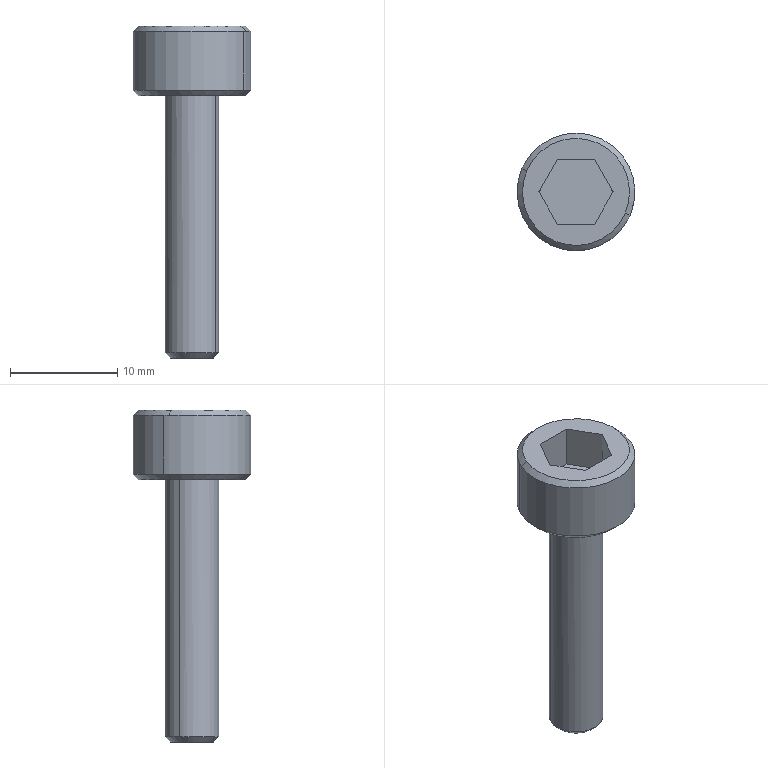Part | STEP file | Bolt.12A.stp | 1 solid | 20 faces | box 11 x 11 x 31 mm | volume 963.854 mm3 | plane 10 | cone 6 | cylinder 4 | commonest cylinder face diameters 5 x2 11 x2
STEP:
#1=CARTESIAN_POINT('',(0.,0.,0.));
#2=DIRECTION('',(0.,0.,1.));
#3=DIRECTION('',(1.,0.,0.));
#4=AXIS2_PLACEMENT_3D('',#1,#2,#3);
#5=CARTESIAN_POINT('',(3.464,0.,0.));
#6=VERTEX_POINT('',#5);
#7=CARTESIAN_POINT('',(3.464,0.,-4.));
#8=VERTEX_POINT('',#7);
#9=CARTESIAN_POINT('',(3.464,0.,0.));
#10=DIRECTION('',(0.,0.,-1.));
#11=VECTOR('',#10,1.);
#12=LINE('',#9,#11);
#13=CARTESIAN_POINT('',(3.551,-0.15,0.2));
#14=DIRECTION('',(-0.866,-0.5,0.));
#15=DIRECTION('',(-0.5,0.866,0.));
#16=AXIS2_PLACEMENT_3D('',#13,#14,#15);
#17=PLANE('',#16);
#18=CARTESIAN_POINT('',(0.1732,0.2));
#19=DIRECTION('',(0.,1.));
#20=VECTOR('',#19,1.);
#21=LINE('',#18,#20);
#22=(GEOMETRIC_REPRESENTATION_CONTEXT(2)PARAMETRIC_REPRESENTATION_CONTEXT()REPRESENTATION_CONTEXT('',''));
#23=DEFINITIONAL_REPRESENTATION('',(#21),#22);
#24=PCURVE('',#17,#23);
#25=CARTESIAN_POINT('',(1.645,-3.15,-4.2));
#26=DIRECTION('',(-0.866,0.5,0.));
#27=DIRECTION('',(0.,0.,1.));
#28=AXIS2_PLACEMENT_3D('',#25,#26,#27);
#29=PLANE('',#28);
#30=CARTESIAN_POINT('',(4.2,3.637));
#31=DIRECTION('',(-1.,0.));
#32=VECTOR('',#31,1.);
#33=LINE('',#30,#32);
#34=(GEOMETRIC_REPRESENTATION_CONTEXT(2)PARAMETRIC_REPRESENTATION_CONTEXT()REPRESENTATION_CONTEXT('',''));
#35=DEFINITIONAL_REPRESENTATION('',(#33),#34);
#36=PCURVE('',#29,#35);
#37=SURFACE_CURVE('',#12,(#24,#36),.PCURVE_S1.);
#38=EDGE_CURVE('',#6,#8,#37,.T.);
#39=ORIENTED_EDGE('',*,*,#38,.F.);
#40=CARTESIAN_POINT('',(1.732,3.,0.));
#41=VERTEX_POINT('',#40);
#42=CARTESIAN_POINT('',(3.464,0.,0.));
#43=DIRECTION('',(-0.5,0.866,0.));
#44=VECTOR('',#43,1.);
#45=LINE('',#42,#44);
#46=CARTESIAN_POINT('',(0.1732,0.2));
#47=DIRECTION('',(1.,0.));
#48=VECTOR('',#47,1.);
#49=LINE('',#46,#48);
#50=(GEOMETRIC_REPRESENTATION_CONTEXT(2)PARAMETRIC_REPRESENTATION_CONTEXT()REPRESENTATION_CONTEXT('',''));
#51=DEFINITIONAL_REPRESENTATION('',(#49),#50);
#52=PCURVE('',#17,#51);
#53=CARTESIAN_POINT('',(5.5,5.5,0.));
#54=DIRECTION('',(0.,0.,-1.));
#55=DIRECTION('',(0.,-1.,0.));
#56=AXIS2_PLACEMENT_3D('',#53,#54,#55);
#57=PLANE('',#56);
#58=CARTESIAN_POINT('',(5.5,2.036));
#59=DIRECTION('',(-0.866,0.5));
#60=VECTOR('',#59,1.);
#61=LINE('',#58,#60);
#62=(GEOMETRIC_REPRESENTATION_CONTEXT(2)PARAMETRIC_REPRESENTATION_CONTEXT()REPRESENTATION_CONTEXT('',''));
#63=DEFINITIONAL_REPRESENTATION('',(#61),#62);
#64=PCURVE('',#57,#63);
#65=SURFACE_CURVE('',#45,(#52,#64),.PCURVE_S1.);
#66=EDGE_CURVE('',#6,#41,#65,.T.);
#67=ORIENTED_EDGE('',*,*,#66,.T.);
#68=CARTESIAN_POINT('',(1.732,3.,-4.));
#69=VERTEX_POINT('',#68);
#70=CARTESIAN_POINT('',(1.732,3.,0.));
#71=DIRECTION('',(0.,0.,-1.));
#72=VECTOR('',#71,1.);
#73=LINE('',#70,#72);
#74=CARTESIAN_POINT('',(3.637,0.2));
#75=DIRECTION('',(0.,1.));
#76=VECTOR('',#75,1.);
#77=LINE('',#74,#76);
#78=(GEOMETRIC_REPRESENTATION_CONTEXT(2)PARAMETRIC_REPRESENTATION_CONTEXT()REPRESENTATION_CONTEXT('',''));
#79=DEFINITIONAL_REPRESENTATION('',(#77),#78);
#80=PCURVE('',#17,#79);
#81=CARTESIAN_POINT('',(-1.905,3.,0.2));
#82=DIRECTION('',(0.,-1.,0.));
#83=DIRECTION('',(0.,0.,-1.));
#84=AXIS2_PLACEMENT_3D('',#81,#82,#83);
#85=PLANE('',#84);
#86=CARTESIAN_POINT('',(0.2,3.637));
#87=DIRECTION('',(1.,0.));
#88=VECTOR('',#87,1.);
#89=LINE('',#86,#88);
#90=(GEOMETRIC_REPRESENTATION_CONTEXT(2)PARAMETRIC_REPRESENTATION_CONTEXT()REPRESENTATION_CONTEXT('',''));
#91=DEFINITIONAL_REPRESENTATION('',(#89),#90);
#92=PCURVE('',#85,#91);
#93=SURFACE_CURVE('',#73,(#80,#92),.PCURVE_S1.);
#94=EDGE_CURVE('',#41,#69,#93,.T.);
#95=ORIENTED_EDGE('',*,*,#94,.T.);
#96=CARTESIAN_POINT('',(3.464,0.,-4.));
#97=DIRECTION('',(-0.5,0.866,0.));
#98=VECTOR('',#97,1.);
#99=LINE('',#96,#98);
#100=CARTESIAN_POINT('',(0.1732,4.2));
#101=DIRECTION('',(1.,0.));
#102=VECTOR('',#101,1.);
#103=LINE('',#100,#102);
#104=(GEOMETRIC_REPRESENTATION_CONTEXT(2)PARAMETRIC_REPRESENTATION_CONTEXT()REPRESENTATION_CONTEXT('',''));
#105=DEFINITIONAL_REPRESENTATION('',(#103),#104);
#106=PCURVE('',#17,#105);
#107=CARTESIAN_POINT('',(-3.811,-3.3,-4.));
#108=DIRECTION('',(0.,0.,1.));
#109=DIRECTION('',(1.,0.,0.));
#110=AXIS2_PLACEMENT_3D('',#107,#108,#109);
#111=PLANE('',#110);
#112=CARTESIAN_POINT('',(7.275,3.3));
#113=DIRECTION('',(-0.5,0.866));
#114=VECTOR('',#113,1.);
#115=LINE('',#112,#114);
#116=(GEOMETRIC_REPRESENTATION_CONTEXT(2)PARAMETRIC_REPRESENTATION_CONTEXT()REPRESENTATION_CONTEXT('',''));
#117=DEFINITIONAL_REPRESENTATION('',(#115),#116);
#118=PCURVE('',#111,#117);
#119=SURFACE_CURVE('',#99,(#106,#118),.PCURVE_S1.);
#120=EDGE_CURVE('',#8,#69,#119,.T.);
#121=ORIENTED_EDGE('',*,*,#120,.F.);
#122=EDGE_LOOP('',(#39,#67,#95,#121));
#123=FACE_BOUND('',#122,.T.);
#124=ADVANCED_FACE('',(#123),#17,.T.);
#125=CARTESIAN_POINT('',(-1.732,3.,0.));
#126=VERTEX_POINT('',#125);
#127=CARTESIAN_POINT('',(-1.732,3.,-4.));
#128=VERTEX_POINT('',#127);
#129=CARTESIAN_POINT('',(-1.732,3.,0.));
#130=DIRECTION('',(0.,0.,-1.));
#131=VECTOR('',#130,1.);
#132=LINE('',#129,#131);
#133=CARTESIAN_POINT('',(-3.551,-0.15,0.2));
#134=DIRECTION('',(0.866,-0.5,0.));
#135=DIRECTION('',(0.,0.,-1.));
#136=AXIS2_PLACEMENT_3D('',#133,#134,#135);
#137=PLANE('',#136);
#138=CARTESIAN_POINT('',(0.2,3.637));
#139=DIRECTION('',(1.,0.));
#140=VECTOR('',#139,1.);
#141=LINE('',#138,#140);
#142=(GEOMETRIC_REPRESENTATION_CONTEXT(2)PARAMETRIC_REPRESENTATION_CONTEXT()REPRESENTATION_CONTEXT('',''));
#143=DEFINITIONAL_REPRESENTATION('',(#141),#142);
#144=PCURVE('',#137,#143);
#145=CARTESIAN_POINT('',(0.2,0.1732));
#146=DIRECTION('',(1.,0.));
#147=VECTOR('',#146,1.);
#148=LINE('',#145,#147);
#149=(GEOMETRIC_REPRESENTATION_CONTEXT(2)PARAMETRIC_REPRESENTATION_CONTEXT()REPRESENTATION_CONTEXT('',''));
#150=DEFINITIONAL_REPRESENTATION('',(#148),#149);
#151=PCURVE('',#85,#150);
#152=SURFACE_CURVE('',#132,(#144,#151),.PCURVE_S1.);
#153=EDGE_CURVE('',#126,#128,#152,.T.);
#154=ORIENTED_EDGE('',*,*,#153,.F.);
#155=CARTESIAN_POINT('',(-3.464,0.,0.));
#156=VERTEX_POINT('',#155);
#157=CARTESIAN_POINT('',(-1.732,3.,0.));
#158=DIRECTION('',(-0.5,-0.866,0.));
#159=VECTOR('',#158,1.);
#160=LINE('',#157,#159);
#161=CARTESIAN_POINT('',(0.2,3.637));
#162=DIRECTION('',(0.,-1.));
#163=VECTOR('',#162,1.);
#164=LINE('',#161,#163);
#165=(GEOMETRIC_REPRESENTATION_CONTEXT(2)PARAMETRIC_REPRESENTATION_CONTEXT()REPRESENTATION_CONTEXT('',''));
#166=DEFINITIONAL_REPRESENTATION('',(#164),#165);
#167=PCURVE('',#137,#166);
#168=CARTESIAN_POINT('',(2.5,7.232));
#169=DIRECTION('',(0.866,0.5));
#170=VECTOR('',#169,1.);
#171=LINE('',#168,#170);
#172=(GEOMETRIC_REPRESENTATION_CONTEXT(2)PARAMETRIC_REPRESENTATION_CONTEXT()REPRESENTATION_CONTEXT('',''));
#173=DEFINITIONAL_REPRESENTATION('',(#171),#172);
#174=PCURVE('',#57,#173);
#175=SURFACE_CURVE('',#160,(#167,#174),.PCURVE_S1.);
#176=EDGE_CURVE('',#126,#156,#175,.T.);
#177=ORIENTED_EDGE('',*,*,#176,.T.);
#178=CARTESIAN_POINT('',(-3.464,0.,-4.));
#179=VERTEX_POINT('',#178);
#180=CARTESIAN_POINT('',(-3.464,0.,0.));
#181=DIRECTION('',(0.,0.,-1.));
#182=VECTOR('',#181,1.);
#183=LINE('',#180,#182);
#184=CARTESIAN_POINT('',(0.2,0.1732));
#185=DIRECTION('',(1.,0.));
#186=VECTOR('',#185,1.);
#187=LINE('',#184,#186);
#188=(GEOMETRIC_REPRESENTATION_CONTEXT(2)PARAMETRIC_REPRESENTATION_CONTEXT()REPRESENTATION_CONTEXT('',''));
#189=DEFINITIONAL_REPRESENTATION('',(#187),#188);
#190=PCURVE('',#137,#189);
#191=CARTESIAN_POINT('',(-1.645,-3.15,0.2));
#192=DIRECTION('',(0.866,0.5,0.));
#193=DIRECTION('',(0.,0.,-1.));
#194=AXIS2_PLACEMENT_3D('',#191,#192,#193);
#195=PLANE('',#194);
#196=CARTESIAN_POINT('',(0.2,3.637));
#197=DIRECTION('',(1.,0.));
#198=VECTOR('',#197,1.);
#199=LINE('',#196,#198);
#200=(GEOMETRIC_REPRESENTATION_CONTEXT(2)PARAMETRIC_REPRESENTATION_CONTEXT()REPRESENTATION_CONTEXT('',''));
#201=DEFINITIONAL_REPRESENTATION('',(#199),#200);
#202=PCURVE('',#195,#201);
#203=SURFACE_CURVE('',#183,(#190,#202),.PCURVE_S1.);
#204=EDGE_CURVE('',#156,#179,#203,.T.);
#205=ORIENTED_EDGE('',*,*,#204,.T.);
#206=CARTESIAN_POINT('',(-1.732,3.,-4.));
#207=DIRECTION('',(-0.5,-0.866,0.));
#208=VECTOR('',#207,1.);
#209=LINE('',#206,#208);
#210=CARTESIAN_POINT('',(4.2,3.637));
#211=DIRECTION('',(0.,-1.));
#212=VECTOR('',#211,1.);
#213=LINE('',#210,#212);
#214=(GEOMETRIC_REPRESENTATION_CONTEXT(2)PARAMETRIC_REPRESENTATION_CONTEXT()REPRESENTATION_CONTEXT('',''));
#215=DEFINITIONAL_REPRESENTATION('',(#213),#214);
#216=PCURVE('',#137,#215);
#217=CARTESIAN_POINT('',(2.078,6.3));
#218=DIRECTION('',(-0.5,-0.866));
#219=VECTOR('',#218,1.);
#220=LINE('',#217,#219);
#221=(GEOMETRIC_REPRESENTATION_CONTEXT(2)PARAMETRIC_REPRESENTATION_CONTEXT()REPRESENTATION_CONTEXT('',''));
#222=DEFINITIONAL_REPRESENTATION('',(#220),#221);
#223=PCURVE('',#111,#222);
#224=SURFACE_CURVE('',#209,(#216,#223),.PCURVE_S1.);
#225=EDGE_CURVE('',#128,#179,#224,.T.);
#226=ORIENTED_EDGE('',*,*,#225,.F.);
#227=EDGE_LOOP('',(#154,#177,#205,#226));
#228=FACE_BOUND('',#227,.T.);
#229=ADVANCED_FACE('',(#228),#137,.T.);
#230=CARTESIAN_POINT('',(-1.732,-3.,-4.));
#231=VERTEX_POINT('',#230);
#232=CARTESIAN_POINT('',(1.732,-3.,-4.));
#233=VERTEX_POINT('',#232);
#234=CARTESIAN_POINT('',(-1.732,-3.,-4.));
#235=DIRECTION('',(1.,0.,0.));
#236=VECTOR('',#235,1.);
#237=LINE('',#234,#236);
#238=CARTESIAN_POINT('',(2.078,0.3));
#239=DIRECTION('',(1.,0.));
#240=VECTOR('',#239,1.);
#241=LINE('',#238,#240);
#242=(GEOMETRIC_REPRESENTATION_CONTEXT(2)PARAMETRIC_REPRESENTATION_CONTEXT()REPRESENTATION_CONTEXT('',''));
#243=DEFINITIONAL_REPRESENTATION('',(#241),#242);
#244=PCURVE('',#111,#243);
#245=CARTESIAN_POINT('',(-1.905,-3.,0.2));
#246=DIRECTION('',(0.,1.,0.));
#247=DIRECTION('',(1.,0.,0.));
#248=AXIS2_PLACEMENT_3D('',#245,#246,#247);
#249=PLANE('',#248);
#250=CARTESIAN_POINT('',(0.1732,4.2));
#251=DIRECTION('',(1.,0.));
#252=VECTOR('',#251,1.);
#253=LINE('',#250,#252);
#254=(GEOMETRIC_REPRESENTATION_CONTEXT(2)PARAMETRIC_REPRESENTATION_CONTEXT()REPRESENTATION_CONTEXT('',''));
#255=DEFINITIONAL_REPRESENTATION('',(#253),#254);
#256=PCURVE('',#249,#255);
#257=SURFACE_CURVE('',#237,(#244,#256),.PCURVE_S1.);
#258=EDGE_CURVE('',#231,#233,#257,.T.);
#259=ORIENTED_EDGE('',*,*,#258,.T.);
#260=CARTESIAN_POINT('',(1.732,-3.,-4.));
#261=DIRECTION('',(0.5,0.866,0.));
#262=VECTOR('',#261,1.);
#263=LINE('',#260,#262);
#264=CARTESIAN_POINT('',(5.543,0.3));
#265=DIRECTION('',(0.5,0.866));
#266=VECTOR('',#265,1.);
#267=LINE('',#264,#266);
#268=(GEOMETRIC_REPRESENTATION_CONTEXT(2)PARAMETRIC_REPRESENTATION_CONTEXT()REPRESENTATION_CONTEXT('',''));
#269=DEFINITIONAL_REPRESENTATION('',(#267),#268);
#270=PCURVE('',#111,#269);
#271=CARTESIAN_POINT('',(0.2,0.1732));
#272=DIRECTION('',(0.,1.));
#273=VECTOR('',#272,1.);
#274=LINE('',#271,#273);
#275=(GEOMETRIC_REPRESENTATION_CONTEXT(2)PARAMETRIC_REPRESENTATION_CONTEXT()REPRESENTATION_CONTEXT('',''));
#276=DEFINITIONAL_REPRESENTATION('',(#274),#275);
#277=PCURVE('',#29,#276);
#278=SURFACE_CURVE('',#263,(#270,#277),.PCURVE_S1.);
#279=EDGE_CURVE('',#233,#8,#278,.T.);
#280=ORIENTED_EDGE('',*,*,#279,.T.);
#281=ORIENTED_EDGE('',*,*,#120,.T.);
#282=CARTESIAN_POINT('',(1.732,3.,-4.));
#283=DIRECTION('',(-1.,0.,0.));
#284=VECTOR('',#283,1.);
#285=LINE('',#282,#284);
#286=CARTESIAN_POINT('',(5.543,6.3));
#287=DIRECTION('',(-1.,0.));
#288=VECTOR('',#287,1.);
#289=LINE('',#286,#288);
#290=(GEOMETRIC_REPRESENTATION_CONTEXT(2)PARAMETRIC_REPRESENTATION_CONTEXT()REPRESENTATION_CONTEXT('',''));
#291=DEFINITIONAL_REPRESENTATION('',(#289),#290);
#292=PCURVE('',#111,#291);
#293=CARTESIAN_POINT('',(4.2,3.637));
#294=DIRECTION('',(0.,-1.));
#295=VECTOR('',#294,1.);
#296=LINE('',#293,#295);
#297=(GEOMETRIC_REPRESENTATION_CONTEXT(2)PARAMETRIC_REPRESENTATION_CONTEXT()REPRESENTATION_CONTEXT('',''));
#298=DEFINITIONAL_REPRESENTATION('',(#296),#297);
#299=PCURVE('',#85,#298);
#300=SURFACE_CURVE('',#285,(#292,#299),.PCURVE_S1.);
#301=EDGE_CURVE('',#69,#128,#300,.T.);
#302=ORIENTED_EDGE('',*,*,#301,.T.);
#303=ORIENTED_EDGE('',*,*,#225,.T.);
#304=CARTESIAN_POINT('',(-3.464,0.,-4.));
#305=DIRECTION('',(0.5,-0.866,0.));
#306=VECTOR('',#305,1.);
#307=LINE('',#304,#306);
#308=CARTESIAN_POINT('',(0.3464,3.3));
#309=DIRECTION('',(0.5,-0.866));
#310=VECTOR('',#309,1.);
#311=LINE('',#308,#310);
#312=(GEOMETRIC_REPRESENTATION_CONTEXT(2)PARAMETRIC_REPRESENTATION_CONTEXT()REPRESENTATION_CONTEXT('',''));
#313=DEFINITIONAL_REPRESENTATION('',(#311),#312);
#314=PCURVE('',#111,#313);
#315=CARTESIAN_POINT('',(4.2,3.637));
#316=DIRECTION('',(0.,-1.));
#317=VECTOR('',#316,1.);
#318=LINE('',#315,#317);
#319=(GEOMETRIC_REPRESENTATION_CONTEXT(2)PARAMETRIC_REPRESENTATION_CONTEXT()REPRESENTATION_CONTEXT('',''));
#320=DEFINITIONAL_REPRESENTATION('',(#318),#319);
#321=PCURVE('',#195,#320);
#322=SURFACE_CURVE('',#307,(#314,#321),.PCURVE_S1.);
#323=EDGE_CURVE('',#179,#231,#322,.T.);
#324=ORIENTED_EDGE('',*,*,#323,.T.);
#325=EDGE_LOOP('',(#259,#280,#281,#302,#303,#324));
#326=FACE_BOUND('',#325,.T.);
#327=ADVANCED_FACE('',(#326),#111,.T.);
#328=CARTESIAN_POINT('',(1.732,-3.,0.));
#329=VERTEX_POINT('',#328);
#330=CARTESIAN_POINT('',(1.732,-3.,0.));
#331=DIRECTION('',(0.,0.,-1.));
#332=VECTOR('',#331,1.);
#333=LINE('',#330,#332);
#334=CARTESIAN_POINT('',(4.2,0.1732));
#335=DIRECTION('',(-1.,0.));
#336=VECTOR('',#335,1.);
#337=LINE('',#334,#336);
#338=(GEOMETRIC_REPRESENTATION_CONTEXT(2)PARAMETRIC_REPRESENTATION_CONTEXT()REPRESENTATION_CONTEXT('',''));
#339=DEFINITIONAL_REPRESENTATION('',(#337),#338);
#340=PCURVE('',#29,#339);
#341=CARTESIAN_POINT('',(3.637,0.2));
#342=DIRECTION('',(0.,1.));
#343=VECTOR('',#342,1.);
#344=LINE('',#341,#343);
#345=(GEOMETRIC_REPRESENTATION_CONTEXT(2)PARAMETRIC_REPRESENTATION_CONTEXT()REPRESENTATION_CONTEXT('',''));
#346=DEFINITIONAL_REPRESENTATION('',(#344),#345);
#347=PCURVE('',#249,#346);
#348=SURFACE_CURVE('',#333,(#340,#347),.PCURVE_S1.);
#349=EDGE_CURVE('',#329,#233,#348,.T.);
#350=ORIENTED_EDGE('',*,*,#349,.F.);
#351=CARTESIAN_POINT('',(1.732,-3.,0.));
#352=DIRECTION('',(0.5,0.866,0.));
#353=VECTOR('',#352,1.);
#354=LINE('',#351,#353);
#355=CARTESIAN_POINT('',(4.2,0.1732));
#356=DIRECTION('',(0.,1.));
#357=VECTOR('',#356,1.);
#358=LINE('',#355,#357);
#359=(GEOMETRIC_REPRESENTATION_CONTEXT(2)PARAMETRIC_REPRESENTATION_CONTEXT()REPRESENTATION_CONTEXT('',''));
#360=DEFINITIONAL_REPRESENTATION('',(#358),#359);
#361=PCURVE('',#29,#360);
#362=CARTESIAN_POINT('',(8.5,3.768));
#363=DIRECTION('',(-0.866,-0.5));
#364=VECTOR('',#363,1.);
#365=LINE('',#362,#364);
#366=(GEOMETRIC_REPRESENTATION_CONTEXT(2)PARAMETRIC_REPRESENTATION_CONTEXT()REPRESENTATION_CONTEXT('',''));
#367=DEFINITIONAL_REPRESENTATION('',(#365),#366);
#368=PCURVE('',#57,#367);
#369=SURFACE_CURVE('',#354,(#361,#368),.PCURVE_S1.);
#370=EDGE_CURVE('',#329,#6,#369,.T.);
#371=ORIENTED_EDGE('',*,*,#370,.T.);
#372=ORIENTED_EDGE('',*,*,#38,.T.);
#373=ORIENTED_EDGE('',*,*,#279,.F.);
#374=EDGE_LOOP('',(#350,#371,#372,#373));
#375=FACE_BOUND('',#374,.T.);
#376=ADVANCED_FACE('',(#375),#29,.T.);
#377=CARTESIAN_POINT('',(2.194,-1.199,-6.5));
#378=VERTEX_POINT('',#377);
#379=CARTESIAN_POINT('',(-2.194,1.199,-6.5));
#380=VERTEX_POINT('',#379);
#381=CARTESIAN_POINT('',(0.,0.,-6.5));
#382=DIRECTION('',(0.,0.,-1.));
#383=DIRECTION('',(1.,0.,0.));
#384=AXIS2_PLACEMENT_3D('',#381,#382,#383);
#385=CIRCLE('',#384,2.5);
#386=CARTESIAN_POINT('',(5.5,5.5,-6.5));
#387=DIRECTION('',(0.,0.,-1.));
#388=DIRECTION('',(0.,-1.,0.));
#389=AXIS2_PLACEMENT_3D('',#386,#387,#388);
#390=PLANE('',#389);
#391=CARTESIAN_POINT('',(5.5,5.5));
#392=DIRECTION('',(0.,-1.));
#393=AXIS2_PLACEMENT_2D('',#391,#392);
#394=CIRCLE('',#393,2.5);
#395=(GEOMETRIC_REPRESENTATION_CONTEXT(2)PARAMETRIC_REPRESENTATION_CONTEXT()REPRESENTATION_CONTEXT('',''));
#396=DEFINITIONAL_REPRESENTATION('',(#394),#395);
#397=PCURVE('',#390,#396);
#398=CARTESIAN_POINT('',(0.,0.,-5.3));
#399=DIRECTION('',(0.,0.,-1.));
#400=DIRECTION('',(0.8776,-0.4794,0.));
#401=AXIS2_PLACEMENT_3D('',#398,#399,#400);
#402=CYLINDRICAL_SURFACE('',#401,2.5);
#403=CARTESIAN_POINT('',(-0.5,1.2));
#404=DIRECTION('',(1.,0.));
#405=VECTOR('',#404,1.);
#406=LINE('',#403,#405);
#407=(GEOMETRIC_REPRESENTATION_CONTEXT(2)PARAMETRIC_REPRESENTATION_CONTEXT()REPRESENTATION_CONTEXT('',''));
#408=DEFINITIONAL_REPRESENTATION('',(#406),#407);
#409=PCURVE('',#402,#408);
#410=SURFACE_CURVE('',#385,(#397,#409),.PCURVE_S1.);
#411=EDGE_CURVE('',#378,#380,#410,.T.);
#412=ORIENTED_EDGE('',*,*,#411,.F.);
#413=CARTESIAN_POINT('',(0.,0.,-6.5));
#414=DIRECTION('',(0.,0.,-1.));
#415=DIRECTION('',(1.,0.,0.));
#416=AXIS2_PLACEMENT_3D('',#413,#414,#415);
#417=CIRCLE('',#416,2.5);
#418=CARTESIAN_POINT('',(5.5,5.5));
#419=DIRECTION('',(0.,-1.));
#420=AXIS2_PLACEMENT_2D('',#418,#419);
#421=CIRCLE('',#420,2.5);
#422=(GEOMETRIC_REPRESENTATION_CONTEXT(2)PARAMETRIC_REPRESENTATION_CONTEXT()REPRESENTATION_CONTEXT('',''));
#423=DEFINITIONAL_REPRESENTATION('',(#421),#422);
#424=PCURVE('',#390,#423);
#425=CARTESIAN_POINT('',(0.,0.,-5.3));
#426=DIRECTION('',(0.,0.,-1.));
#427=DIRECTION('',(0.8776,-0.4794,0.));
#428=AXIS2_PLACEMENT_3D('',#425,#426,#427);
#429=CYLINDRICAL_SURFACE('',#428,2.5);
#430=CARTESIAN_POINT('',(-0.5,1.2));
#431=DIRECTION('',(1.,0.));
#432=VECTOR('',#431,1.);
#433=LINE('',#430,#432);
#434=(GEOMETRIC_REPRESENTATION_CONTEXT(2)PARAMETRIC_REPRESENTATION_CONTEXT()REPRESENTATION_CONTEXT('',''));
#435=DEFINITIONAL_REPRESENTATION('',(#433),#434);
#436=PCURVE('',#429,#435);
#437=SURFACE_CURVE('',#417,(#424,#436),.PCURVE_S1.);
#438=EDGE_CURVE('',#380,#378,#437,.T.);
#439=ORIENTED_EDGE('',*,*,#438,.F.);
#440=EDGE_LOOP('',(#412,#439));
#441=FACE_BOUND('',#440,.T.);
#442=CARTESIAN_POINT('',(-4.597,1.967,-6.5));
#443=VERTEX_POINT('',#442);
#444=CARTESIAN_POINT('',(4.597,-1.967,-6.5));
#445=VERTEX_POINT('',#444);
#446=CARTESIAN_POINT('',(0.,0.,-6.5));
#447=DIRECTION('',(0.,0.,-1.));
#448=DIRECTION('',(1.,0.,0.));
#449=AXIS2_PLACEMENT_3D('',#446,#447,#448);
#450=CIRCLE('',#449,5.);
#451=CARTESIAN_POINT('',(5.5,5.5));
#452=DIRECTION('',(0.,-1.));
#453=AXIS2_PLACEMENT_2D('',#451,#452);
#454=CIRCLE('',#453,5.);
#455=(GEOMETRIC_REPRESENTATION_CONTEXT(2)PARAMETRIC_REPRESENTATION_CONTEXT()REPRESENTATION_CONTEXT('',''));
#456=DEFINITIONAL_REPRESENTATION('',(#454),#455);
#457=PCURVE('',#390,#456);
#458=CARTESIAN_POINT('',(0.,0.,-6.525));
#459=DIRECTION('',(0.,0.,1.));
#460=DIRECTION('',(-0.9193,0.3935,0.));
#461=AXIS2_PLACEMENT_3D('',#458,#459,#460);
#462=CONICAL_SURFACE('',#461,4.975,0.7854);
#463=CARTESIAN_POINT('',(9.829,0.025));
#464=DIRECTION('',(-1.,0.));
#465=VECTOR('',#464,1.);
#466=LINE('',#463,#465);
#467=(GEOMETRIC_REPRESENTATION_CONTEXT(2)PARAMETRIC_REPRESENTATION_CONTEXT()REPRESENTATION_CONTEXT('',''));
#468=DEFINITIONAL_REPRESENTATION('',(#466),#467);
#469=PCURVE('',#462,#468);
#470=SURFACE_CURVE('',#450,(#457,#469),.PCURVE_S1.);
#471=EDGE_CURVE('',#443,#445,#470,.T.);
#472=ORIENTED_EDGE('',*,*,#471,.T.);
#473=CARTESIAN_POINT('',(0.,0.,-6.5));
#474=DIRECTION('',(0.,0.,-1.));
#475=DIRECTION('',(1.,0.,0.));
#476=AXIS2_PLACEMENT_3D('',#473,#474,#475);
#477=CIRCLE('',#476,5.);
#478=CARTESIAN_POINT('',(5.5,5.5));
#479=DIRECTION('',(0.,-1.));
#480=AXIS2_PLACEMENT_2D('',#478,#479);
#481=CIRCLE('',#480,5.);
#482=(GEOMETRIC_REPRESENTATION_CONTEXT(2)PARAMETRIC_REPRESENTATION_CONTEXT()REPRESENTATION_CONTEXT('',''));
#483=DEFINITIONAL_REPRESENTATION('',(#481),#482);
#484=PCURVE('',#390,#483);
#485=CARTESIAN_POINT('',(0.,0.,-6.525));
#486=DIRECTION('',(0.,0.,1.));
#487=DIRECTION('',(-0.9193,0.3935,0.));
#488=AXIS2_PLACEMENT_3D('',#485,#486,#487);
#489=CONICAL_SURFACE('',#488,4.975,0.7854);
#490=CARTESIAN_POINT('',(3.546,0.025));
#491=DIRECTION('',(-1.,0.));
#492=VECTOR('',#491,1.);
#493=LINE('',#490,#492);
#494=(GEOMETRIC_REPRESENTATION_CONTEXT(2)PARAMETRIC_REPRESENTATION_CONTEXT()REPRESENTATION_CONTEXT('',''));
#495=DEFINITIONAL_REPRESENTATION('',(#493),#494);
#496=PCURVE('',#489,#495);
#497=SURFACE_CURVE('',#477,(#484,#496),.PCURVE_S1.);
#498=EDGE_CURVE('',#445,#443,#497,.T.);
#499=ORIENTED_EDGE('',*,*,#498,.T.);
#500=EDGE_LOOP('',(#472,#499));
#501=FACE_BOUND('',#500,.T.);
#502=ADVANCED_FACE('',(#441,#501),#390,.T.);
#503=CARTESIAN_POINT('',(-5.056,2.164,-6.));
#504=VERTEX_POINT('',#503);
#505=CARTESIAN_POINT('',(-5.056,2.164,-6.));
#506=DIRECTION('',(0.6501,-0.2782,-0.7071));
#507=VECTOR('',#506,1.);
#508=LINE('',#505,#507);
#509=CARTESIAN_POINT('',(0.,0.525));
#510=DIRECTION('',(0.,-1.));
#511=VECTOR('',#510,1.);
#512=LINE('',#509,#511);
#513=(GEOMETRIC_REPRESENTATION_CONTEXT(2)PARAMETRIC_REPRESENTATION_CONTEXT()REPRESENTATION_CONTEXT('',''));
#514=DEFINITIONAL_REPRESENTATION('',(#512),#513);
#515=PCURVE('',#489,#514);
#516=CARTESIAN_POINT('',(6.283,0.525));
#517=DIRECTION('',(0.,-1.));
#518=VECTOR('',#517,1.);
#519=LINE('',#516,#518);
#520=(GEOMETRIC_REPRESENTATION_CONTEXT(2)PARAMETRIC_REPRESENTATION_CONTEXT()REPRESENTATION_CONTEXT('',''));
#521=DEFINITIONAL_REPRESENTATION('',(#519),#520);
#522=PCURVE('',#462,#521);
#523=SURFACE_CURVE('',#508,(#515,#522),.PCURVE_S1.);
#524=EDGE_CURVE('',#504,#443,#523,.T.);
#525=ORIENTED_EDGE('',*,*,#524,.T.);
#526=ORIENTED_EDGE('',*,*,#498,.F.);
#527=CARTESIAN_POINT('',(5.056,-2.164,-6.));
#528=VERTEX_POINT('',#527);
#529=CARTESIAN_POINT('',(5.056,-2.164,-6.));
#530=DIRECTION('',(-0.6501,0.2782,-0.7071));
#531=VECTOR('',#530,1.);
#532=LINE('',#529,#531);
#533=CARTESIAN_POINT('',(3.142,0.525));
#534=DIRECTION('',(0.,-1.));
#535=VECTOR('',#534,1.);
#536=LINE('',#533,#535);
#537=(GEOMETRIC_REPRESENTATION_CONTEXT(2)PARAMETRIC_REPRESENTATION_CONTEXT()REPRESENTATION_CONTEXT('',''));
#538=DEFINITIONAL_REPRESENTATION('',(#536),#537);
#539=PCURVE('',#489,#538);
#540=CARTESIAN_POINT('',(3.142,0.525));
#541=DIRECTION('',(0.,-1.));
#542=VECTOR('',#541,1.);
#543=LINE('',#540,#542);
#544=(GEOMETRIC_REPRESENTATION_CONTEXT(2)PARAMETRIC_REPRESENTATION_CONTEXT()REPRESENTATION_CONTEXT('',''));
#545=DEFINITIONAL_REPRESENTATION('',(#543),#544);
#546=PCURVE('',#462,#545);
#547=SURFACE_CURVE('',#532,(#539,#546),.PCURVE_S1.);
#548=EDGE_CURVE('',#528,#445,#547,.T.);
#549=ORIENTED_EDGE('',*,*,#548,.F.);
#550=CARTESIAN_POINT('',(4.827,-2.637,-6.));
#551=VERTEX_POINT('',#550);
#552=CARTESIAN_POINT('',(0.,0.,-6.));
#553=DIRECTION('',(0.,0.,-1.));
#554=DIRECTION('',(1.,0.,0.));
#555=AXIS2_PLACEMENT_3D('',#552,#553,#554);
#556=CIRCLE('',#555,5.5);
#557=CARTESIAN_POINT('',(3.546,0.525));
#558=DIRECTION('',(-1.,0.));
#559=VECTOR('',#558,1.);
#560=LINE('',#557,#559);
#561=(GEOMETRIC_REPRESENTATION_CONTEXT(2)PARAMETRIC_REPRESENTATION_CONTEXT()REPRESENTATION_CONTEXT('',''));
#562=DEFINITIONAL_REPRESENTATION('',(#560),#561);
#563=PCURVE('',#489,#562);
#564=CARTESIAN_POINT('',(0.,0.,-0.225));
#565=DIRECTION('',(0.,0.,-1.));
#566=DIRECTION('',(0.8776,-0.4794,0.));
#567=AXIS2_PLACEMENT_3D('',#564,#565,#566);
#568=CYLINDRICAL_SURFACE('',#567,5.5);
#569=CARTESIAN_POINT('',(5.783,5.775));
#570=DIRECTION('',(1.,0.));
#571=VECTOR('',#570,1.);
#572=LINE('',#569,#571);
#573=(GEOMETRIC_REPRESENTATION_CONTEXT(2)PARAMETRIC_REPRESENTATION_CONTEXT()REPRESENTATION_CONTEXT('',''));
#574=DEFINITIONAL_REPRESENTATION('',(#572),#573);
#575=PCURVE('',#568,#574);
#576=SURFACE_CURVE('',#556,(#563,#575),.PCURVE_S1.);
#577=EDGE_CURVE('',#528,#551,#576,.T.);
#578=ORIENTED_EDGE('',*,*,#577,.T.);
#579=CARTESIAN_POINT('',(0.,0.,-6.));
#580=DIRECTION('',(0.,0.,-1.));
#581=DIRECTION('',(1.,0.,0.));
#582=AXIS2_PLACEMENT_3D('',#579,#580,#581);
#583=CIRCLE('',#582,5.5);
#584=CARTESIAN_POINT('',(3.546,0.525));
#585=DIRECTION('',(-1.,0.));
#586=VECTOR('',#585,1.);
#587=LINE('',#584,#586);
#588=(GEOMETRIC_REPRESENTATION_CONTEXT(2)PARAMETRIC_REPRESENTATION_CONTEXT()REPRESENTATION_CONTEXT('',''));
#589=DEFINITIONAL_REPRESENTATION('',(#587),#588);
#590=PCURVE('',#489,#589);
#591=CARTESIAN_POINT('',(0.,0.,-0.225));
#592=DIRECTION('',(0.,0.,-1.));
#593=DIRECTION('',(0.8776,-0.4794,0.));
#594=AXIS2_PLACEMENT_3D('',#591,#592,#593);
#595=CYLINDRICAL_SURFACE('',#594,5.5);
#596=CARTESIAN_POINT('',(-0.5,5.775));
#597=DIRECTION('',(1.,0.));
#598=VECTOR('',#597,1.);
#599=LINE('',#596,#598);
#600=(GEOMETRIC_REPRESENTATION_CONTEXT(2)PARAMETRIC_REPRESENTATION_CONTEXT()REPRESENTATION_CONTEXT('',''));
#601=DEFINITIONAL_REPRESENTATION('',(#599),#600);
#602=PCURVE('',#595,#601);
#603=SURFACE_CURVE('',#583,(#590,#602),.PCURVE_S1.);
#604=EDGE_CURVE('',#551,#504,#603,.T.);
#605=ORIENTED_EDGE('',*,*,#604,.T.);
#606=EDGE_LOOP('',(#525,#526,#549,#578,#605));
#607=FACE_BOUND('',#606,.T.);
#608=ADVANCED_FACE('',(#607),#489,.T.);
#609=CARTESIAN_POINT('',(4.827,-2.637,-0.5));
#610=VERTEX_POINT('',#609);
#611=CARTESIAN_POINT('',(4.827,-2.637,-6.));
#612=DIRECTION('',(0.,0.,1.));
#613=VECTOR('',#612,1.);
#614=LINE('',#611,#613);
#615=CARTESIAN_POINT('',(0.,5.775));
#616=DIRECTION('',(0.,-1.));
#617=VECTOR('',#616,1.);
#618=LINE('',#615,#617);
#619=(GEOMETRIC_REPRESENTATION_CONTEXT(2)PARAMETRIC_REPRESENTATION_CONTEXT()REPRESENTATION_CONTEXT('',''));
#620=DEFINITIONAL_REPRESENTATION('',(#618),#619);
#621=PCURVE('',#595,#620);
#622=CARTESIAN_POINT('',(6.283,5.775));
#623=DIRECTION('',(0.,-1.));
#624=VECTOR('',#623,1.);
#625=LINE('',#622,#624);
#626=(GEOMETRIC_REPRESENTATION_CONTEXT(2)PARAMETRIC_REPRESENTATION_CONTEXT()REPRESENTATION_CONTEXT('',''));
#627=DEFINITIONAL_REPRESENTATION('',(#625),#626);
#628=PCURVE('',#568,#627);
#629=SURFACE_CURVE('',#614,(#621,#628),.PCURVE_S1.);
#630=EDGE_CURVE('',#551,#610,#629,.T.);
#631=ORIENTED_EDGE('',*,*,#630,.T.);
#632=CARTESIAN_POINT('',(-5.056,2.164,-0.5));
#633=VERTEX_POINT('',#632);
#634=CARTESIAN_POINT('',(0.,0.,-0.5));
#635=DIRECTION('',(0.,0.,-1.));
#636=DIRECTION('',(1.,0.,0.));
#637=AXIS2_PLACEMENT_3D('',#634,#635,#636);
#638=CIRCLE('',#637,5.5);
#639=CARTESIAN_POINT('',(-0.5,0.275));
#640=DIRECTION('',(1.,0.));
#641=VECTOR('',#640,1.);
#642=LINE('',#639,#641);
#643=(GEOMETRIC_REPRESENTATION_CONTEXT(2)PARAMETRIC_REPRESENTATION_CONTEXT()REPRESENTATION_CONTEXT('',''));
#644=DEFINITIONAL_REPRESENTATION('',(#642),#643);
#645=PCURVE('',#595,#644);
#646=CARTESIAN_POINT('',(0.,0.,0.025));
#647=DIRECTION('',(0.,0.,-1.));
#648=DIRECTION('',(-0.9193,0.3935,0.));
#649=AXIS2_PLACEMENT_3D('',#646,#647,#648);
#650=CONICAL_SURFACE('',#649,4.975,0.7854);
#651=CARTESIAN_POINT('',(2.737,0.525));
#652=DIRECTION('',(1.,0.));
#653=VECTOR('',#652,1.);
#654=LINE('',#651,#653);
#655=(GEOMETRIC_REPRESENTATION_CONTEXT(2)PARAMETRIC_REPRESENTATION_CONTEXT()REPRESENTATION_CONTEXT('',''));
#656=DEFINITIONAL_REPRESENTATION('',(#654),#655);
#657=PCURVE('',#650,#656);
#658=SURFACE_CURVE('',#638,(#645,#657),.PCURVE_S1.);
#659=EDGE_CURVE('',#610,#633,#658,.T.);
#660=ORIENTED_EDGE('',*,*,#659,.T.);
#661=CARTESIAN_POINT('',(-4.827,2.637,-0.5));
#662=VERTEX_POINT('',#661);
#663=CARTESIAN_POINT('',(0.,0.,-0.5));
#664=DIRECTION('',(0.,0.,-1.));
#665=DIRECTION('',(1.,0.,0.));
#666=AXIS2_PLACEMENT_3D('',#663,#664,#665);
#667=CIRCLE('',#666,5.5);
#668=CARTESIAN_POINT('',(-0.5,0.275));
#669=DIRECTION('',(1.,0.));
#670=VECTOR('',#669,1.);
#671=LINE('',#668,#670);
#672=(GEOMETRIC_REPRESENTATION_CONTEXT(2)PARAMETRIC_REPRESENTATION_CONTEXT()REPRESENTATION_CONTEXT('',''));
#673=DEFINITIONAL_REPRESENTATION('',(#671),#672);
#674=PCURVE('',#595,#673);
#675=CARTESIAN_POINT('',(0.,0.,0.025));
#676=DIRECTION('',(0.,0.,-1.));
#677=DIRECTION('',(-0.9193,0.3935,0.));
#678=AXIS2_PLACEMENT_3D('',#675,#676,#677);
#679=CONICAL_SURFACE('',#678,4.975,0.7854);
#680=CARTESIAN_POINT('',(-3.546,0.525));
#681=DIRECTION('',(1.,0.));
#682=VECTOR('',#681,1.);
#683=LINE('',#680,#682);
#684=(GEOMETRIC_REPRESENTATION_CONTEXT(2)PARAMETRIC_REPRESENTATION_CONTEXT()REPRESENTATION_CONTEXT('',''));
#685=DEFINITIONAL_REPRESENTATION('',(#683),#684);
#686=PCURVE('',#679,#685);
#687=SURFACE_CURVE('',#667,(#674,#686),.PCURVE_S1.);
#688=EDGE_CURVE('',#633,#662,#687,.T.);
#689=ORIENTED_EDGE('',*,*,#688,.T.);
#690=CARTESIAN_POINT('',(-4.827,2.637,-6.));
#691=VERTEX_POINT('',#690);
#692=CARTESIAN_POINT('',(-4.827,2.637,-6.));
#693=DIRECTION('',(0.,0.,1.));
#694=VECTOR('',#693,1.);
#695=LINE('',#692,#694);
#696=CARTESIAN_POINT('',(3.142,5.775));
#697=DIRECTION('',(0.,-1.));
#698=VECTOR('',#697,1.);
#699=LINE('',#696,#698);
#700=(GEOMETRIC_REPRESENTATION_CONTEXT(2)PARAMETRIC_REPRESENTATION_CONTEXT()REPRESENTATION_CONTEXT('',''));
#701=DEFINITIONAL_REPRESENTATION('',(#699),#700);
#702=PCURVE('',#595,#701);
#703=CARTESIAN_POINT('',(3.142,5.775));
#704=DIRECTION('',(0.,-1.));
#705=VECTOR('',#704,1.);
#706=LINE('',#703,#705);
#707=(GEOMETRIC_REPRESENTATION_CONTEXT(2)PARAMETRIC_REPRESENTATION_CONTEXT()REPRESENTATION_CONTEXT('',''));
#708=DEFINITIONAL_REPRESENTATION('',(#706),#707);
#709=PCURVE('',#568,#708);
#710=SURFACE_CURVE('',#695,(#702,#709),.PCURVE_S1.);
#711=EDGE_CURVE('',#691,#662,#710,.T.);
#712=ORIENTED_EDGE('',*,*,#711,.F.);
#713=CARTESIAN_POINT('',(0.,0.,-6.));
#714=DIRECTION('',(0.,0.,-1.));
#715=DIRECTION('',(1.,0.,0.));
#716=AXIS2_PLACEMENT_3D('',#713,#714,#715);
#717=CIRCLE('',#716,5.5);
#718=CARTESIAN_POINT('',(-0.5,5.775));
#719=DIRECTION('',(1.,0.));
#720=VECTOR('',#719,1.);
#721=LINE('',#718,#720);
#722=(GEOMETRIC_REPRESENTATION_CONTEXT(2)PARAMETRIC_REPRESENTATION_CONTEXT()REPRESENTATION_CONTEXT('',''));
#723=DEFINITIONAL_REPRESENTATION('',(#721),#722);
#724=PCURVE('',#595,#723);
#725=CARTESIAN_POINT('',(9.829,0.525));
#726=DIRECTION('',(-1.,0.));
#727=VECTOR('',#726,1.);
#728=LINE('',#725,#727);
#729=(GEOMETRIC_REPRESENTATION_CONTEXT(2)PARAMETRIC_REPRESENTATION_CONTEXT()REPRESENTATION_CONTEXT('',''));
#730=DEFINITIONAL_REPRESENTATION('',(#728),#729);
#731=PCURVE('',#462,#730);
#732=SURFACE_CURVE('',#717,(#724,#731),.PCURVE_S1.);
#733=EDGE_CURVE('',#504,#691,#732,.T.);
#734=ORIENTED_EDGE('',*,*,#733,.F.);
#735=ORIENTED_EDGE('',*,*,#604,.F.);
#736=EDGE_LOOP('',(#631,#660,#689,#712,#734,#735));
#737=FACE_BOUND('',#736,.T.);
#738=ADVANCED_FACE('',(#737),#595,.T.);
#739=CARTESIAN_POINT('',(-2.455,0.4718,-30.5));
#740=VERTEX_POINT('',#739);
#741=CARTESIAN_POINT('',(-1.964,0.3775,-31.));
#742=VERTEX_POINT('',#741);
#743=CARTESIAN_POINT('',(-2.455,0.4718,-30.5));
#744=DIRECTION('',(0.6944,-0.1335,-0.7071));
#745=VECTOR('',#744,1.);
#746=LINE('',#743,#745);
#747=CARTESIAN_POINT('',(0.,0.,-31.025));
#748=DIRECTION('',(0.,0.,1.));
#749=DIRECTION('',(-0.982,0.1887,0.));
#750=AXIS2_PLACEMENT_3D('',#747,#748,#749);
#751=CONICAL_SURFACE('',#750,1.975,0.7854);
#752=CARTESIAN_POINT('',(0.,0.525));
#753=DIRECTION('',(0.,-1.));
#754=VECTOR('',#753,1.);
#755=LINE('',#752,#754);
#756=(GEOMETRIC_REPRESENTATION_CONTEXT(2)PARAMETRIC_REPRESENTATION_CONTEXT()REPRESENTATION_CONTEXT('',''));
#757=DEFINITIONAL_REPRESENTATION('',(#755),#756);
#758=PCURVE('',#751,#757);
#759=CARTESIAN_POINT('',(0.,0.,-31.025));
#760=DIRECTION('',(0.,0.,1.));
#761=DIRECTION('',(-0.982,0.1887,0.));
#762=AXIS2_PLACEMENT_3D('',#759,#760,#761);
#763=CONICAL_SURFACE('',#762,1.975,0.7854);
#764=CARTESIAN_POINT('',(6.283,0.525));
#765=DIRECTION('',(0.,-1.));
#766=VECTOR('',#765,1.);
#767=LINE('',#764,#766);
#768=(GEOMETRIC_REPRESENTATION_CONTEXT(2)PARAMETRIC_REPRESENTATION_CONTEXT()REPRESENTATION_CONTEXT('',''));
#769=DEFINITIONAL_REPRESENTATION('',(#767),#768);
#770=PCURVE('',#763,#769);
#771=SURFACE_CURVE('',#746,(#758,#770),.PCURVE_S1.);
#772=EDGE_CURVE('',#740,#742,#771,.T.);
#773=ORIENTED_EDGE('',*,*,#772,.T.);
#774=CARTESIAN_POINT('',(1.964,-0.3775,-31.));
#775=VERTEX_POINT('',#774);
#776=CARTESIAN_POINT('',(0.,0.,-31.));
#777=DIRECTION('',(0.,0.,-1.));
#778=DIRECTION('',(1.,0.,0.));
#779=AXIS2_PLACEMENT_3D('',#776,#777,#778);
#780=CIRCLE('',#779,2.);
#781=CARTESIAN_POINT('',(3.331,0.025));
#782=DIRECTION('',(-1.,0.));
#783=VECTOR('',#782,1.);
#784=LINE('',#781,#783);
#785=(GEOMETRIC_REPRESENTATION_CONTEXT(2)PARAMETRIC_REPRESENTATION_CONTEXT()REPRESENTATION_CONTEXT('',''));
#786=DEFINITIONAL_REPRESENTATION('',(#784),#785);
#787=PCURVE('',#751,#786);
#788=CARTESIAN_POINT('',(2.2,2.2,-31.));
#789=DIRECTION('',(0.,0.,-1.));
#790=DIRECTION('',(0.,-1.,0.));
#791=AXIS2_PLACEMENT_3D('',#788,#789,#790);
#792=PLANE('',#791);
#793=CARTESIAN_POINT('',(2.2,2.2));
#794=DIRECTION('',(0.,-1.));
#795=AXIS2_PLACEMENT_2D('',#793,#794);
#796=CIRCLE('',#795,2.);
#797=(GEOMETRIC_REPRESENTATION_CONTEXT(2)PARAMETRIC_REPRESENTATION_CONTEXT()REPRESENTATION_CONTEXT('',''));
#798=DEFINITIONAL_REPRESENTATION('',(#796),#797);
#799=PCURVE('',#792,#798);
#800=SURFACE_CURVE('',#780,(#787,#799),.PCURVE_S1.);
#801=EDGE_CURVE('',#775,#742,#800,.T.);
#802=ORIENTED_EDGE('',*,*,#801,.F.);
#803=CARTESIAN_POINT('',(2.455,-0.4718,-30.5));
#804=VERTEX_POINT('',#803);
#805=CARTESIAN_POINT('',(2.455,-0.4718,-30.5));
#806=DIRECTION('',(-0.6944,0.1335,-0.7071));
#807=VECTOR('',#806,1.);
#808=LINE('',#805,#807);
#809=CARTESIAN_POINT('',(3.142,0.525));
#810=DIRECTION('',(0.,-1.));
#811=VECTOR('',#810,1.);
#812=LINE('',#809,#811);
#813=(GEOMETRIC_REPRESENTATION_CONTEXT(2)PARAMETRIC_REPRESENTATION_CONTEXT()REPRESENTATION_CONTEXT('',''));
#814=DEFINITIONAL_REPRESENTATION('',(#812),#813);
#815=PCURVE('',#751,#814);
#816=CARTESIAN_POINT('',(3.142,0.525));
#817=DIRECTION('',(0.,-1.));
#818=VECTOR('',#817,1.);
#819=LINE('',#816,#818);
#820=(GEOMETRIC_REPRESENTATION_CONTEXT(2)PARAMETRIC_REPRESENTATION_CONTEXT()REPRESENTATION_CONTEXT('',''));
#821=DEFINITIONAL_REPRESENTATION('',(#819),#820);
#822=PCURVE('',#763,#821);
#823=SURFACE_CURVE('',#808,(#815,#822),.PCURVE_S1.);
#824=EDGE_CURVE('',#804,#775,#823,.T.);
#825=ORIENTED_EDGE('',*,*,#824,.F.);
#826=CARTESIAN_POINT('',(2.194,-1.199,-30.5));
#827=VERTEX_POINT('',#826);
#828=CARTESIAN_POINT('',(0.,0.,-30.5));
#829=DIRECTION('',(0.,0.,-1.));
#830=DIRECTION('',(1.,0.,0.));
#831=AXIS2_PLACEMENT_3D('',#828,#829,#830);
#832=CIRCLE('',#831,2.5);
#833=CARTESIAN_POINT('',(3.331,0.525));
#834=DIRECTION('',(-1.,0.));
#835=VECTOR('',#834,1.);
#836=LINE('',#833,#835);
#837=(GEOMETRIC_REPRESENTATION_CONTEXT(2)PARAMETRIC_REPRESENTATION_CONTEXT()REPRESENTATION_CONTEXT('',''));
#838=DEFINITIONAL_REPRESENTATION('',(#836),#837);
#839=PCURVE('',#751,#838);
#840=CARTESIAN_POINT('',(5.783,25.2));
#841=DIRECTION('',(1.,0.));
#842=VECTOR('',#841,1.);
#843=LINE('',#840,#842);
#844=(GEOMETRIC_REPRESENTATION_CONTEXT(2)PARAMETRIC_REPRESENTATION_CONTEXT()REPRESENTATION_CONTEXT('',''));
#845=DEFINITIONAL_REPRESENTATION('',(#843),#844);
#846=PCURVE('',#429,#845);
#847=SURFACE_CURVE('',#832,(#839,#846),.PCURVE_S1.);
#848=EDGE_CURVE('',#804,#827,#847,.T.);
#849=ORIENTED_EDGE('',*,*,#848,.T.);
#850=CARTESIAN_POINT('',(0.,0.,-30.5));
#851=DIRECTION('',(0.,0.,-1.));
#852=DIRECTION('',(1.,0.,0.));
#853=AXIS2_PLACEMENT_3D('',#850,#851,#852);
#854=CIRCLE('',#853,2.5);
#855=CARTESIAN_POINT('',(3.331,0.525));
#856=DIRECTION('',(-1.,0.));
#857=VECTOR('',#856,1.);
#858=LINE('',#855,#857);
#859=(GEOMETRIC_REPRESENTATION_CONTEXT(2)PARAMETRIC_REPRESENTATION_CONTEXT()REPRESENTATION_CONTEXT('',''));
#860=DEFINITIONAL_REPRESENTATION('',(#858),#859);
#861=PCURVE('',#751,#860);
#862=CARTESIAN_POINT('',(-0.5,25.2));
#863=DIRECTION('',(1.,0.));
#864=VECTOR('',#863,1.);
#865=LINE('',#862,#864);
#866=(GEOMETRIC_REPRESENTATION_CONTEXT(2)PARAMETRIC_REPRESENTATION_CONTEXT()REPRESENTATION_CONTEXT('',''));
#867=DEFINITIONAL_REPRESENTATION('',(#865),#866);
#868=PCURVE('',#402,#867);
#869=SURFACE_CURVE('',#854,(#861,#868),.PCURVE_S1.);
#870=EDGE_CURVE('',#827,#740,#869,.T.);
#871=ORIENTED_EDGE('',*,*,#870,.T.);
#872=EDGE_LOOP('',(#773,#802,#825,#849,#871));
#873=FACE_BOUND('',#872,.T.);
#874=ADVANCED_FACE('',(#873),#751,.T.);
#875=CARTESIAN_POINT('',(0.,0.,-31.));
#876=DIRECTION('',(0.,0.,-1.));
#877=DIRECTION('',(1.,0.,0.));
#878=AXIS2_PLACEMENT_3D('',#875,#876,#877);
#879=CIRCLE('',#878,2.);
#880=CARTESIAN_POINT('',(2.2,2.2));
#881=DIRECTION('',(0.,-1.));
#882=AXIS2_PLACEMENT_2D('',#880,#881);
#883=CIRCLE('',#882,2.);
#884=(GEOMETRIC_REPRESENTATION_CONTEXT(2)PARAMETRIC_REPRESENTATION_CONTEXT()REPRESENTATION_CONTEXT('',''));
#885=DEFINITIONAL_REPRESENTATION('',(#883),#884);
#886=PCURVE('',#792,#885);
#887=CARTESIAN_POINT('',(9.615,0.025));
#888=DIRECTION('',(-1.,0.));
#889=VECTOR('',#888,1.);
#890=LINE('',#887,#889);
#891=(GEOMETRIC_REPRESENTATION_CONTEXT(2)PARAMETRIC_REPRESENTATION_CONTEXT()REPRESENTATION_CONTEXT('',''));
#892=DEFINITIONAL_REPRESENTATION('',(#890),#891);
#893=PCURVE('',#763,#892);
#894=SURFACE_CURVE('',#879,(#886,#893),.PCURVE_S1.);
#895=EDGE_CURVE('',#742,#775,#894,.T.);
#896=ORIENTED_EDGE('',*,*,#895,.T.);
#897=ORIENTED_EDGE('',*,*,#801,.T.);
#898=EDGE_LOOP('',(#896,#897));
#899=FACE_BOUND('',#898,.T.);
#900=ADVANCED_FACE('',(#899),#792,.T.);
#901=CARTESIAN_POINT('',(2.194,-1.199,-30.5));
#902=DIRECTION('',(0.,0.,1.));
#903=VECTOR('',#902,1.);
#904=LINE('',#901,#903);
#905=CARTESIAN_POINT('',(0.,25.2));
#906=DIRECTION('',(0.,-1.));
#907=VECTOR('',#906,1.);
#908=LINE('',#905,#907);
#909=(GEOMETRIC_REPRESENTATION_CONTEXT(2)PARAMETRIC_REPRESENTATION_CONTEXT()REPRESENTATION_CONTEXT('',''));
#910=DEFINITIONAL_REPRESENTATION('',(#908),#909);
#911=PCURVE('',#402,#910);
#912=CARTESIAN_POINT('',(6.283,25.2));
#913=DIRECTION('',(0.,-1.));
#914=VECTOR('',#913,1.);
#915=LINE('',#912,#914);
#916=(GEOMETRIC_REPRESENTATION_CONTEXT(2)PARAMETRIC_REPRESENTATION_CONTEXT()REPRESENTATION_CONTEXT('',''));
#917=DEFINITIONAL_REPRESENTATION('',(#915),#916);
#918=PCURVE('',#429,#917);
#919=SURFACE_CURVE('',#904,(#911,#918),.PCURVE_S1.);
#920=EDGE_CURVE('',#827,#378,#919,.T.);
#921=ORIENTED_EDGE('',*,*,#920,.T.);
#922=ORIENTED_EDGE('',*,*,#411,.T.);
#923=CARTESIAN_POINT('',(-2.194,1.199,-30.5));
#924=VERTEX_POINT('',#923);
#925=CARTESIAN_POINT('',(-2.194,1.199,-30.5));
#926=DIRECTION('',(0.,0.,1.));
#927=VECTOR('',#926,1.);
#928=LINE('',#925,#927);
#929=CARTESIAN_POINT('',(3.142,25.2));
#930=DIRECTION('',(0.,-1.));
#931=VECTOR('',#930,1.);
#932=LINE('',#929,#931);
#933=(GEOMETRIC_REPRESENTATION_CONTEXT(2)PARAMETRIC_REPRESENTATION_CONTEXT()REPRESENTATION_CONTEXT('',''));
#934=DEFINITIONAL_REPRESENTATION('',(#932),#933);
#935=PCURVE('',#402,#934);
#936=CARTESIAN_POINT('',(3.142,25.2));
#937=DIRECTION('',(0.,-1.));
#938=VECTOR('',#937,1.);
#939=LINE('',#936,#938);
#940=(GEOMETRIC_REPRESENTATION_CONTEXT(2)PARAMETRIC_REPRESENTATION_CONTEXT()REPRESENTATION_CONTEXT('',''));
#941=DEFINITIONAL_REPRESENTATION('',(#939),#940);
#942=PCURVE('',#429,#941);
#943=SURFACE_CURVE('',#928,(#935,#942),.PCURVE_S1.);
#944=EDGE_CURVE('',#924,#380,#943,.T.);
#945=ORIENTED_EDGE('',*,*,#944,.F.);
#946=CARTESIAN_POINT('',(0.,0.,-30.5));
#947=DIRECTION('',(0.,0.,-1.));
#948=DIRECTION('',(1.,0.,0.));
#949=AXIS2_PLACEMENT_3D('',#946,#947,#948);
#950=CIRCLE('',#949,2.5);
#951=CARTESIAN_POINT('',(-0.5,25.2));
#952=DIRECTION('',(1.,0.));
#953=VECTOR('',#952,1.);
#954=LINE('',#951,#953);
#955=(GEOMETRIC_REPRESENTATION_CONTEXT(2)PARAMETRIC_REPRESENTATION_CONTEXT()REPRESENTATION_CONTEXT('',''));
#956=DEFINITIONAL_REPRESENTATION('',(#954),#955);
#957=PCURVE('',#402,#956);
#958=CARTESIAN_POINT('',(9.615,0.525));
#959=DIRECTION('',(-1.,0.));
#960=VECTOR('',#959,1.);
#961=LINE('',#958,#960);
#962=(GEOMETRIC_REPRESENTATION_CONTEXT(2)PARAMETRIC_REPRESENTATION_CONTEXT()REPRESENTATION_CONTEXT('',''));
#963=DEFINITIONAL_REPRESENTATION('',(#961),#962);
#964=PCURVE('',#763,#963);
#965=SURFACE_CURVE('',#950,(#957,#964),.PCURVE_S1.);
#966=EDGE_CURVE('',#740,#924,#965,.T.);
#967=ORIENTED_EDGE('',*,*,#966,.F.);
#968=ORIENTED_EDGE('',*,*,#870,.F.);
#969=EDGE_LOOP('',(#921,#922,#945,#967,#968));
#970=FACE_BOUND('',#969,.T.);
#971=ADVANCED_FACE('',(#970),#402,.T.);
#972=ORIENTED_EDGE('',*,*,#204,.F.);
#973=CARTESIAN_POINT('',(-1.732,-3.,0.));
#974=VERTEX_POINT('',#973);
#975=CARTESIAN_POINT('',(-3.464,0.,0.));
#976=DIRECTION('',(0.5,-0.866,0.));
#977=VECTOR('',#976,1.);
#978=LINE('',#975,#977);
#979=CARTESIAN_POINT('',(0.2,3.637));
#980=DIRECTION('',(0.,-1.));
#981=VECTOR('',#980,1.);
#982=LINE('',#979,#981);
#983=(GEOMETRIC_REPRESENTATION_CONTEXT(2)PARAMETRIC_REPRESENTATION_CONTEXT()REPRESENTATION_CONTEXT('',''));
#984=DEFINITIONAL_REPRESENTATION('',(#982),#983);
#985=PCURVE('',#195,#984);
#986=CARTESIAN_POINT('',(5.5,8.964));
#987=DIRECTION('',(0.866,-0.5));
#988=VECTOR('',#987,1.);
#989=LINE('',#986,#988);
#990=(GEOMETRIC_REPRESENTATION_CONTEXT(2)PARAMETRIC_REPRESENTATION_CONTEXT()REPRESENTATION_CONTEXT('',''));
#991=DEFINITIONAL_REPRESENTATION('',(#989),#990);
#992=PCURVE('',#57,#991);
#993=SURFACE_CURVE('',#978,(#985,#992),.PCURVE_S1.);
#994=EDGE_CURVE('',#156,#974,#993,.T.);
#995=ORIENTED_EDGE('',*,*,#994,.T.);
#996=CARTESIAN_POINT('',(-1.732,-3.,0.));
#997=DIRECTION('',(0.,0.,-1.));
#998=VECTOR('',#997,1.);
#999=LINE('',#996,#998);
#1000=CARTESIAN_POINT('',(0.2,0.1732));
#1001=DIRECTION('',(1.,0.));
#1002=VECTOR('',#1001,1.);
#1003=LINE('',#1000,#1002);
#1004=(GEOMETRIC_REPRESENTATION_CONTEXT(2)PARAMETRIC_REPRESENTATION_CONTEXT()REPRESENTATION_CONTEXT('',''));
#1005=DEFINITIONAL_REPRESENTATION('',(#1003),#1004);
#1006=PCURVE('',#195,#1005);
#1007=CARTESIAN_POINT('',(0.1732,0.2));
#1008=DIRECTION('',(0.,1.));
#1009=VECTOR('',#1008,1.);
#1010=LINE('',#1007,#1009);
#1011=(GEOMETRIC_REPRESENTATION_CONTEXT(2)PARAMETRIC_REPRESENTATION_CONTEXT()REPRESENTATION_CONTEXT('',''));
#1012=DEFINITIONAL_REPRESENTATION('',(#1010),#1011);
#1013=PCURVE('',#249,#1012);
#1014=SURFACE_CURVE('',#999,(#1006,#1013),.PCURVE_S1.);
#1015=EDGE_CURVE('',#974,#231,#1014,.T.);
#1016=ORIENTED_EDGE('',*,*,#1015,.T.);
#1017=ORIENTED_EDGE('',*,*,#323,.F.);
#1018=EDGE_LOOP('',(#972,#995,#1016,#1017));
#1019=FACE_BOUND('',#1018,.T.);
#1020=ADVANCED_FACE('',(#1019),#195,.T.);
#1021=ORIENTED_EDGE('',*,*,#1015,.F.);
#1022=CARTESIAN_POINT('',(-1.732,-3.,0.));
#1023=DIRECTION('',(1.,0.,0.));
#1024=VECTOR('',#1023,1.);
#1025=LINE('',#1022,#1024);
#1026=CARTESIAN_POINT('',(0.1732,0.2));
#1027=DIRECTION('',(1.,0.));
#1028=VECTOR('',#1027,1.);
#1029=LINE('',#1026,#1028);
#1030=(GEOMETRIC_REPRESENTATION_CONTEXT(2)PARAMETRIC_REPRESENTATION_CONTEXT()REPRESENTATION_CONTEXT('',''));
#1031=DEFINITIONAL_REPRESENTATION('',(#1029),#1030);
#1032=PCURVE('',#249,#1031);
#1033=CARTESIAN_POINT('',(8.5,7.232));
#1034=DIRECTION('',(0.,-1.));
#1035=VECTOR('',#1034,1.);
#1036=LINE('',#1033,#1035);
#1037=(GEOMETRIC_REPRESENTATION_CONTEXT(2)PARAMETRIC_REPRESENTATION_CONTEXT()REPRESENTATION_CONTEXT('',''));
#1038=DEFINITIONAL_REPRESENTATION('',(#1036),#1037);
#1039=PCURVE('',#57,#1038);
#1040=SURFACE_CURVE('',#1025,(#1032,#1039),.PCURVE_S1.);
#1041=EDGE_CURVE('',#974,#329,#1040,.T.);
#1042=ORIENTED_EDGE('',*,*,#1041,.T.);
#1043=ORIENTED_EDGE('',*,*,#349,.T.);
#1044=ORIENTED_EDGE('',*,*,#258,.F.);
#1045=EDGE_LOOP('',(#1021,#1042,#1043,#1044));
#1046=FACE_BOUND('',#1045,.T.);
#1047=ADVANCED_FACE('',(#1046),#249,.T.);
#1048=ORIENTED_EDGE('',*,*,#94,.F.);
#1049=CARTESIAN_POINT('',(1.732,3.,0.));
#1050=DIRECTION('',(-1.,0.,0.));
#1051=VECTOR('',#1050,1.);
#1052=LINE('',#1049,#1051);
#1053=CARTESIAN_POINT('',(0.2,3.637));
#1054=DIRECTION('',(0.,-1.));
#1055=VECTOR('',#1054,1.);
#1056=LINE('',#1053,#1055);
#1057=(GEOMETRIC_REPRESENTATION_CONTEXT(2)PARAMETRIC_REPRESENTATION_CONTEXT()REPRESENTATION_CONTEXT('',''));
#1058=DEFINITIONAL_REPRESENTATION('',(#1056),#1057);
#1059=PCURVE('',#85,#1058);
#1060=CARTESIAN_POINT('',(2.5,3.768));
#1061=DIRECTION('',(0.,1.));
#1062=VECTOR('',#1061,1.);
#1063=LINE('',#1060,#1062);
#1064=(GEOMETRIC_REPRESENTATION_CONTEXT(2)PARAMETRIC_REPRESENTATION_CONTEXT()REPRESENTATION_CONTEXT('',''));
#1065=DEFINITIONAL_REPRESENTATION('',(#1063),#1064);
#1066=PCURVE('',#57,#1065);
#1067=SURFACE_CURVE('',#1052,(#1059,#1066),.PCURVE_S1.);
#1068=EDGE_CURVE('',#41,#126,#1067,.T.);
#1069=ORIENTED_EDGE('',*,*,#1068,.T.);
#1070=ORIENTED_EDGE('',*,*,#153,.T.);
#1071=ORIENTED_EDGE('',*,*,#301,.F.);
#1072=EDGE_LOOP('',(#1048,#1069,#1070,#1071));
#1073=FACE_BOUND('',#1072,.T.);
#1074=ADVANCED_FACE('',(#1073),#85,.T.);
#1075=CARTESIAN_POINT('',(-4.597,1.967,0.));
#1076=VERTEX_POINT('',#1075);
#1077=CARTESIAN_POINT('',(-5.056,2.164,-0.5));
#1078=DIRECTION('',(0.6501,-0.2782,0.7071));
#1079=VECTOR('',#1078,1.);
#1080=LINE('',#1077,#1079);
#1081=CARTESIAN_POINT('',(0.,0.525));
#1082=DIRECTION('',(0.,-1.));
#1083=VECTOR('',#1082,1.);
#1084=LINE('',#1081,#1083);
#1085=(GEOMETRIC_REPRESENTATION_CONTEXT(2)PARAMETRIC_REPRESENTATION_CONTEXT()REPRESENTATION_CONTEXT('',''));
#1086=DEFINITIONAL_REPRESENTATION('',(#1084),#1085);
#1087=PCURVE('',#679,#1086);
#1088=CARTESIAN_POINT('',(6.283,0.525));
#1089=DIRECTION('',(0.,-1.));
#1090=VECTOR('',#1089,1.);
#1091=LINE('',#1088,#1090);
#1092=(GEOMETRIC_REPRESENTATION_CONTEXT(2)PARAMETRIC_REPRESENTATION_CONTEXT()REPRESENTATION_CONTEXT('',''));
#1093=DEFINITIONAL_REPRESENTATION('',(#1091),#1092);
#1094=PCURVE('',#650,#1093);
#1095=SURFACE_CURVE('',#1080,(#1087,#1094),.PCURVE_S1.);
#1096=EDGE_CURVE('',#633,#1076,#1095,.T.);
#1097=ORIENTED_EDGE('',*,*,#1096,.T.);
#1098=CARTESIAN_POINT('',(4.597,-1.967,0.));
#1099=VERTEX_POINT('',#1098);
#1100=CARTESIAN_POINT('',(0.,0.,0.));
#1101=DIRECTION('',(0.,0.,-1.));
#1102=DIRECTION('',(1.,0.,0.));
#1103=AXIS2_PLACEMENT_3D('',#1100,#1101,#1102);
#1104=CIRCLE('',#1103,5.);
#1105=CARTESIAN_POINT('',(-3.546,0.025));
#1106=DIRECTION('',(1.,0.));
#1107=VECTOR('',#1106,1.);
#1108=LINE('',#1105,#1107);
#1109=(GEOMETRIC_REPRESENTATION_CONTEXT(2)PARAMETRIC_REPRESENTATION_CONTEXT()REPRESENTATION_CONTEXT('',''));
#1110=DEFINITIONAL_REPRESENTATION('',(#1108),#1109);
#1111=PCURVE('',#679,#1110);
#1112=CARTESIAN_POINT('',(5.5,5.5));
#1113=DIRECTION('',(0.,-1.));
#1114=AXIS2_PLACEMENT_2D('',#1112,#1113);
#1115=CIRCLE('',#1114,5.);
#1116=(GEOMETRIC_REPRESENTATION_CONTEXT(2)PARAMETRIC_REPRESENTATION_CONTEXT()REPRESENTATION_CONTEXT('',''));
#1117=DEFINITIONAL_REPRESENTATION('',(#1115),#1116);
#1118=PCURVE('',#57,#1117);
#1119=SURFACE_CURVE('',#1104,(#1111,#1118),.PCURVE_S1.);
#1120=EDGE_CURVE('',#1076,#1099,#1119,.T.);
#1121=ORIENTED_EDGE('',*,*,#1120,.T.);
#1122=CARTESIAN_POINT('',(5.056,-2.164,-0.5));
#1123=VERTEX_POINT('',#1122);
#1124=CARTESIAN_POINT('',(5.056,-2.164,-0.5));
#1125=DIRECTION('',(-0.6501,0.2782,0.7071));
#1126=VECTOR('',#1125,1.);
#1127=LINE('',#1124,#1126);
#1128=CARTESIAN_POINT('',(3.142,0.525));
#1129=DIRECTION('',(0.,-1.));
#1130=VECTOR('',#1129,1.);
#1131=LINE('',#1128,#1130);
#1132=(GEOMETRIC_REPRESENTATION_CONTEXT(2)PARAMETRIC_REPRESENTATION_CONTEXT()REPRESENTATION_CONTEXT('',''));
#1133=DEFINITIONAL_REPRESENTATION('',(#1131),#1132);
#1134=PCURVE('',#679,#1133);
#1135=CARTESIAN_POINT('',(3.142,0.525));
#1136=DIRECTION('',(0.,-1.));
#1137=VECTOR('',#1136,1.);
#1138=LINE('',#1135,#1137);
#1139=(GEOMETRIC_REPRESENTATION_CONTEXT(2)PARAMETRIC_REPRESENTATION_CONTEXT()REPRESENTATION_CONTEXT('',''));
#1140=DEFINITIONAL_REPRESENTATION('',(#1138),#1139);
#1141=PCURVE('',#650,#1140);
#1142=SURFACE_CURVE('',#1127,(#1134,#1141),.PCURVE_S1.);
#1143=EDGE_CURVE('',#1123,#1099,#1142,.T.);
#1144=ORIENTED_EDGE('',*,*,#1143,.F.);
#1145=CARTESIAN_POINT('',(0.,0.,-0.5));
#1146=DIRECTION('',(0.,0.,-1.));
#1147=DIRECTION('',(1.,0.,0.));
#1148=AXIS2_PLACEMENT_3D('',#1145,#1146,#1147);
#1149=CIRCLE('',#1148,5.5);
#1150=CARTESIAN_POINT('',(-3.546,0.525));
#1151=DIRECTION('',(1.,0.));
#1152=VECTOR('',#1151,1.);
#1153=LINE('',#1150,#1152);
#1154=(GEOMETRIC_REPRESENTATION_CONTEXT(2)PARAMETRIC_REPRESENTATION_CONTEXT()REPRESENTATION_CONTEXT('',''));
#1155=DEFINITIONAL_REPRESENTATION('',(#1153),#1154);
#1156=PCURVE('',#679,#1155);
#1157=CARTESIAN_POINT('',(-0.5,0.275));
#1158=DIRECTION('',(1.,0.));
#1159=VECTOR('',#1158,1.);
#1160=LINE('',#1157,#1159);
#1161=(GEOMETRIC_REPRESENTATION_CONTEXT(2)PARAMETRIC_REPRESENTATION_CONTEXT()REPRESENTATION_CONTEXT('',''));
#1162=DEFINITIONAL_REPRESENTATION('',(#1160),#1161);
#1163=PCURVE('',#568,#1162);
#1164=SURFACE_CURVE('',#1149,(#1156,#1163),.PCURVE_S1.);
#1165=EDGE_CURVE('',#662,#1123,#1164,.T.);
#1166=ORIENTED_EDGE('',*,*,#1165,.F.);
#1167=ORIENTED_EDGE('',*,*,#688,.F.);
#1168=EDGE_LOOP('',(#1097,#1121,#1144,#1166,#1167));
#1169=FACE_BOUND('',#1168,.T.);
#1170=ADVANCED_FACE('',(#1169),#679,.T.);
#1171=ORIENTED_EDGE('',*,*,#994,.F.);
#1172=ORIENTED_EDGE('',*,*,#176,.F.);
#1173=ORIENTED_EDGE('',*,*,#1068,.F.);
#1174=ORIENTED_EDGE('',*,*,#66,.F.);
#1175=ORIENTED_EDGE('',*,*,#370,.F.);
#1176=ORIENTED_EDGE('',*,*,#1041,.F.);
#1177=EDGE_LOOP('',(#1171,#1172,#1173,#1174,#1175,#1176));
#1178=FACE_BOUND('',#1177,.T.);
#1179=ORIENTED_EDGE('',*,*,#1120,.F.);
#1180=CARTESIAN_POINT('',(0.,0.,0.));
#1181=DIRECTION('',(0.,0.,-1.));
#1182=DIRECTION('',(1.,0.,0.));
#1183=AXIS2_PLACEMENT_3D('',#1180,#1181,#1182);
#1184=CIRCLE('',#1183,5.);
#1185=CARTESIAN_POINT('',(5.5,5.5));
#1186=DIRECTION('',(0.,-1.));
#1187=AXIS2_PLACEMENT_2D('',#1185,#1186);
#1188=CIRCLE('',#1187,5.);
#1189=(GEOMETRIC_REPRESENTATION_CONTEXT(2)PARAMETRIC_REPRESENTATION_CONTEXT()REPRESENTATION_CONTEXT('',''));
#1190=DEFINITIONAL_REPRESENTATION('',(#1188),#1189);
#1191=PCURVE('',#57,#1190);
#1192=CARTESIAN_POINT('',(2.737,0.025));
#1193=DIRECTION('',(1.,0.));
#1194=VECTOR('',#1193,1.);
#1195=LINE('',#1192,#1194);
#1196=(GEOMETRIC_REPRESENTATION_CONTEXT(2)PARAMETRIC_REPRESENTATION_CONTEXT()REPRESENTATION_CONTEXT('',''));
#1197=DEFINITIONAL_REPRESENTATION('',(#1195),#1196);
#1198=PCURVE('',#650,#1197);
#1199=SURFACE_CURVE('',#1184,(#1191,#1198),.PCURVE_S1.);
#1200=EDGE_CURVE('',#1099,#1076,#1199,.T.);
#1201=ORIENTED_EDGE('',*,*,#1200,.F.);
#1202=EDGE_LOOP('',(#1179,#1201));
#1203=FACE_BOUND('',#1202,.T.);
#1204=ADVANCED_FACE('',(#1178,#1203),#57,.F.);
#1205=ORIENTED_EDGE('',*,*,#1096,.F.);
#1206=ORIENTED_EDGE('',*,*,#659,.F.);
#1207=CARTESIAN_POINT('',(0.,0.,-0.5));
#1208=DIRECTION('',(0.,0.,-1.));
#1209=DIRECTION('',(1.,0.,0.));
#1210=AXIS2_PLACEMENT_3D('',#1207,#1208,#1209);
#1211=CIRCLE('',#1210,5.5);
#1212=CARTESIAN_POINT('',(2.737,0.525));
#1213=DIRECTION('',(1.,0.));
#1214=VECTOR('',#1213,1.);
#1215=LINE('',#1212,#1214);
#1216=(GEOMETRIC_REPRESENTATION_CONTEXT(2)PARAMETRIC_REPRESENTATION_CONTEXT()REPRESENTATION_CONTEXT('',''));
#1217=DEFINITIONAL_REPRESENTATION('',(#1215),#1216);
#1218=PCURVE('',#650,#1217);
#1219=CARTESIAN_POINT('',(5.783,0.275));
#1220=DIRECTION('',(1.,0.));
#1221=VECTOR('',#1220,1.);
#1222=LINE('',#1219,#1221);
#1223=(GEOMETRIC_REPRESENTATION_CONTEXT(2)PARAMETRIC_REPRESENTATION_CONTEXT()REPRESENTATION_CONTEXT('',''));
#1224=DEFINITIONAL_REPRESENTATION('',(#1222),#1223);
#1225=PCURVE('',#568,#1224);
#1226=SURFACE_CURVE('',#1211,(#1218,#1225),.PCURVE_S1.);
#1227=EDGE_CURVE('',#1123,#610,#1226,.T.);
#1228=ORIENTED_EDGE('',*,*,#1227,.F.);
#1229=ORIENTED_EDGE('',*,*,#1143,.T.);
#1230=ORIENTED_EDGE('',*,*,#1200,.T.);
#1231=EDGE_LOOP('',(#1205,#1206,#1228,#1229,#1230));
#1232=FACE_BOUND('',#1231,.T.);
#1233=ADVANCED_FACE('',(#1232),#650,.T.);
#1234=ORIENTED_EDGE('',*,*,#920,.F.);
#1235=ORIENTED_EDGE('',*,*,#848,.F.);
#1236=CARTESIAN_POINT('',(0.,0.,-30.5));
#1237=DIRECTION('',(0.,0.,-1.));
#1238=DIRECTION('',(1.,0.,0.));
#1239=AXIS2_PLACEMENT_3D('',#1236,#1237,#1238);
#1240=CIRCLE('',#1239,2.5);
#1241=CARTESIAN_POINT('',(-0.5,25.2));
#1242=DIRECTION('',(1.,0.));
#1243=VECTOR('',#1242,1.);
#1244=LINE('',#1241,#1243);
#1245=(GEOMETRIC_REPRESENTATION_CONTEXT(2)PARAMETRIC_REPRESENTATION_CONTEXT()REPRESENTATION_CONTEXT('',''));
#1246=DEFINITIONAL_REPRESENTATION('',(#1244),#1245);
#1247=PCURVE('',#429,#1246);
#1248=CARTESIAN_POINT('',(9.615,0.525));
#1249=DIRECTION('',(-1.,0.));
#1250=VECTOR('',#1249,1.);
#1251=LINE('',#1248,#1250);
#1252=(GEOMETRIC_REPRESENTATION_CONTEXT(2)PARAMETRIC_REPRESENTATION_CONTEXT()REPRESENTATION_CONTEXT('',''));
#1253=DEFINITIONAL_REPRESENTATION('',(#1251),#1252);
#1254=PCURVE('',#763,#1253);
#1255=SURFACE_CURVE('',#1240,(#1247,#1254),.PCURVE_S1.);
#1256=EDGE_CURVE('',#924,#804,#1255,.T.);
#1257=ORIENTED_EDGE('',*,*,#1256,.F.);
#1258=ORIENTED_EDGE('',*,*,#944,.T.);
#1259=ORIENTED_EDGE('',*,*,#438,.T.);
#1260=EDGE_LOOP('',(#1234,#1235,#1257,#1258,#1259));
#1261=FACE_BOUND('',#1260,.T.);
#1262=ADVANCED_FACE('',(#1261),#429,.T.);
#1263=ORIENTED_EDGE('',*,*,#772,.F.);
#1264=ORIENTED_EDGE('',*,*,#966,.T.);
#1265=ORIENTED_EDGE('',*,*,#1256,.T.);
#1266=ORIENTED_EDGE('',*,*,#824,.T.);
#1267=ORIENTED_EDGE('',*,*,#895,.F.);
#1268=EDGE_LOOP('',(#1263,#1264,#1265,#1266,#1267));
#1269=FACE_BOUND('',#1268,.T.);
#1270=ADVANCED_FACE('',(#1269),#763,.T.);
#1271=ORIENTED_EDGE('',*,*,#630,.F.);
#1272=ORIENTED_EDGE('',*,*,#577,.F.);
#1273=CARTESIAN_POINT('',(0.,0.,-6.));
#1274=DIRECTION('',(0.,0.,-1.));
#1275=DIRECTION('',(1.,0.,0.));
#1276=AXIS2_PLACEMENT_3D('',#1273,#1274,#1275);
#1277=CIRCLE('',#1276,5.5);
#1278=CARTESIAN_POINT('',(-0.5,5.775));
#1279=DIRECTION('',(1.,0.));
#1280=VECTOR('',#1279,1.);
#1281=LINE('',#1278,#1280);
#1282=(GEOMETRIC_REPRESENTATION_CONTEXT(2)PARAMETRIC_REPRESENTATION_CONTEXT()REPRESENTATION_CONTEXT('',''));
#1283=DEFINITIONAL_REPRESENTATION('',(#1281),#1282);
#1284=PCURVE('',#568,#1283);
#1285=CARTESIAN_POINT('',(9.829,0.525));
#1286=DIRECTION('',(-1.,0.));
#1287=VECTOR('',#1286,1.);
#1288=LINE('',#1285,#1287);
#1289=(GEOMETRIC_REPRESENTATION_CONTEXT(2)PARAMETRIC_REPRESENTATION_CONTEXT()REPRESENTATION_CONTEXT('',''));
#1290=DEFINITIONAL_REPRESENTATION('',(#1288),#1289);
#1291=PCURVE('',#462,#1290);
#1292=SURFACE_CURVE('',#1277,(#1284,#1291),.PCURVE_S1.);
#1293=EDGE_CURVE('',#691,#528,#1292,.T.);
#1294=ORIENTED_EDGE('',*,*,#1293,.F.);
#1295=ORIENTED_EDGE('',*,*,#711,.T.);
#1296=ORIENTED_EDGE('',*,*,#1165,.T.);
#1297=ORIENTED_EDGE('',*,*,#1227,.T.);
#1298=EDGE_LOOP('',(#1271,#1272,#1294,#1295,#1296,#1297));
#1299=FACE_BOUND('',#1298,.T.);
#1300=ADVANCED_FACE('',(#1299),#568,.T.);
#1301=ORIENTED_EDGE('',*,*,#524,.F.);
#1302=ORIENTED_EDGE('',*,*,#733,.T.);
#1303=ORIENTED_EDGE('',*,*,#1293,.T.);
#1304=ORIENTED_EDGE('',*,*,#548,.T.);
#1305=ORIENTED_EDGE('',*,*,#471,.F.);
#1306=EDGE_LOOP('',(#1301,#1302,#1303,#1304,#1305));
#1307=FACE_BOUND('',#1306,.T.);
#1308=ADVANCED_FACE('',(#1307),#462,.T.);
#1309=CLOSED_SHELL('',(#124,#229,#327,#376,#502,#608,#738,#874,#900,#971,#1020,#1047,#1074,#1170,#1204,#1233,#1262,#1270,#1300,#1308));
#1310=MANIFOLD_SOLID_BREP('',#1309);
#1311=(LENGTH_UNIT()NAMED_UNIT(*)SI_UNIT(.MILLI.,.METRE.));
#1312=UNCERTAINTY_MEASURE_WITH_UNIT(LENGTH_MEASURE(0.0000001),#1311,'','');
#1313=(NAMED_UNIT(*)PLANE_ANGLE_UNIT()SI_UNIT($,.RADIAN.));
#1314=(NAMED_UNIT(*)SI_UNIT($,.STERADIAN.)SOLID_ANGLE_UNIT());
#1315=(GEOMETRIC_REPRESENTATION_CONTEXT(3)GLOBAL_UNCERTAINTY_ASSIGNED_CONTEXT((#1312))GLOBAL_UNIT_ASSIGNED_CONTEXT((#1311,#1313,#1314))REPRESENTATION_CONTEXT('',''));
#1316=ADVANCED_BREP_SHAPE_REPRESENTATION('',(#4,#1310),#1315);